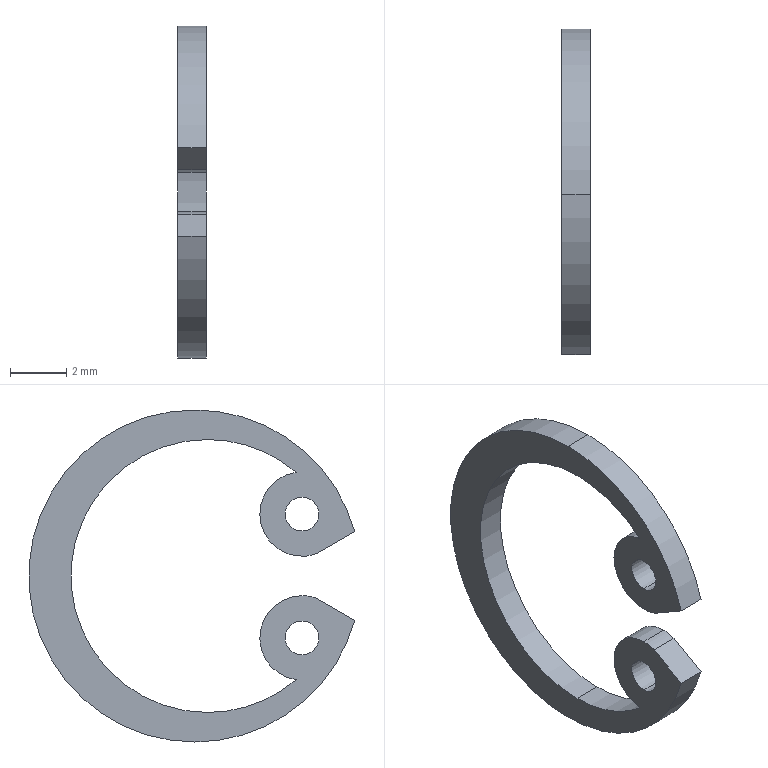Part | SolidWorks | features RefAxis 3, 3DProfileFeature 1, Extrusion 1 | 1 solid | 17 faces | box 1 x 11.586 x 11.8 mm | volume 42.993 mm3 | cylinder 13 | plane 4 | commonest cylinder face diameters 1.2 x4 3 x3 9.7 x3 11.8 x3
STEP:
#1=CARTESIAN_POINT('',(0.5,-3.811,2.8));
#2=VERTEX_POINT('',#1);
#3=CARTESIAN_POINT('',(0.5,-3.811,1.6));
#4=VERTEX_POINT('',#3);
#5=CARTESIAN_POINT('',(0.5,-3.811,2.2));
#6=DIRECTION('',(1.,0.,0.));
#7=DIRECTION('',(0.,0.,-1.));
#8=AXIS2_PLACEMENT_3D('',#5,#6,#7);
#9=CIRCLE('',#8,0.6);
#10=EDGE_CURVE('',#2,#4,#9,.T.);
#11=ORIENTED_EDGE('',*,*,#10,.T.);
#12=CARTESIAN_POINT('',(-0.5,-3.811,1.6));
#13=VERTEX_POINT('',#12);
#14=CARTESIAN_POINT('',(0.5,-3.811,1.6));
#15=DIRECTION('',(-1.,0.,0.));
#16=VECTOR('',#15,1000.);
#17=LINE('',#14,#16);
#18=EDGE_CURVE('',#4,#13,#17,.T.);
#19=ORIENTED_EDGE('',*,*,#18,.T.);
#20=CARTESIAN_POINT('',(-0.5,-3.811,2.8));
#21=VERTEX_POINT('',#20);
#22=CARTESIAN_POINT('',(-0.5,-3.811,2.2));
#23=DIRECTION('',(1.,0.,0.));
#24=DIRECTION('',(0.,0.,-1.));
#25=AXIS2_PLACEMENT_3D('',#22,#23,#24);
#26=CIRCLE('',#25,0.6);
#27=EDGE_CURVE('',#21,#13,#26,.T.);
#28=ORIENTED_EDGE('',*,*,#27,.F.);
#29=CARTESIAN_POINT('',(0.5,-3.811,2.8));
#30=DIRECTION('',(-1.,0.,0.));
#31=VECTOR('',#30,1000.);
#32=LINE('',#29,#31);
#33=EDGE_CURVE('',#2,#21,#32,.T.);
#34=ORIENTED_EDGE('',*,*,#33,.F.);
#35=EDGE_LOOP('',(#11,#19,#28,#34));
#36=FACE_OUTER_BOUND('',#35,.T.);
#37=CARTESIAN_POINT('',(0.5,-3.811,2.2));
#38=DIRECTION('',(-1.,0.,0.));
#39=DIRECTION('',(0.,0.,1.));
#40=AXIS2_PLACEMENT_3D('',#37,#38,#39);
#41=CYLINDRICAL_SURFACE('',#40,0.6);
#42=ADVANCED_FACE('',(#36),#41,.F.);
#43=CARTESIAN_POINT('',(0.5,-3.811,-1.6));
#44=VERTEX_POINT('',#43);
#45=CARTESIAN_POINT('',(0.5,-3.811,-2.8));
#46=VERTEX_POINT('',#45);
#47=CARTESIAN_POINT('',(0.5,-3.811,-2.2));
#48=DIRECTION('',(1.,0.,0.));
#49=DIRECTION('',(0.,0.,-1.));
#50=AXIS2_PLACEMENT_3D('',#47,#48,#49);
#51=CIRCLE('',#50,0.6);
#52=EDGE_CURVE('',#44,#46,#51,.T.);
#53=ORIENTED_EDGE('',*,*,#52,.T.);
#54=CARTESIAN_POINT('',(-0.5,-3.811,-2.8));
#55=VERTEX_POINT('',#54);
#56=CARTESIAN_POINT('',(0.5,-3.811,-2.8));
#57=DIRECTION('',(-1.,0.,0.));
#58=VECTOR('',#57,1000.);
#59=LINE('',#56,#58);
#60=EDGE_CURVE('',#46,#55,#59,.T.);
#61=ORIENTED_EDGE('',*,*,#60,.T.);
#62=CARTESIAN_POINT('',(-0.5,-3.811,-1.6));
#63=VERTEX_POINT('',#62);
#64=CARTESIAN_POINT('',(-0.5,-3.811,-2.2));
#65=DIRECTION('',(1.,0.,0.));
#66=DIRECTION('',(0.,0.,-1.));
#67=AXIS2_PLACEMENT_3D('',#64,#65,#66);
#68=CIRCLE('',#67,0.6);
#69=EDGE_CURVE('',#63,#55,#68,.T.);
#70=ORIENTED_EDGE('',*,*,#69,.F.);
#71=CARTESIAN_POINT('',(0.5,-3.811,-1.6));
#72=DIRECTION('',(-1.,0.,0.));
#73=VECTOR('',#72,1000.);
#74=LINE('',#71,#73);
#75=EDGE_CURVE('',#44,#63,#74,.T.);
#76=ORIENTED_EDGE('',*,*,#75,.F.);
#77=EDGE_LOOP('',(#53,#61,#70,#76));
#78=FACE_OUTER_BOUND('',#77,.T.);
#79=CARTESIAN_POINT('',(0.5,-3.811,-2.2));
#80=DIRECTION('',(-1.,0.,0.));
#81=DIRECTION('',(0.,0.,1.));
#82=AXIS2_PLACEMENT_3D('',#79,#80,#81);
#83=CYLINDRICAL_SURFACE('',#82,0.6);
#84=ADVANCED_FACE('',(#78),#83,.F.);
#85=CARTESIAN_POINT('',(0.5,-3.811,-0.7));
#86=VERTEX_POINT('',#85);
#87=CARTESIAN_POINT('',(0.5,-4.328,-0.7921));
#88=VERTEX_POINT('',#87);
#89=CARTESIAN_POINT('',(0.5,-3.811,-2.2));
#90=DIRECTION('',(1.,0.,0.));
#91=DIRECTION('',(0.,0.,-1.));
#92=AXIS2_PLACEMENT_3D('',#89,#90,#91);
#93=CIRCLE('',#92,1.5);
#94=EDGE_CURVE('',#86,#88,#93,.T.);
#95=ORIENTED_EDGE('',*,*,#94,.F.);
#96=CARTESIAN_POINT('',(-0.5,-3.811,-0.7));
#97=VERTEX_POINT('',#96);
#98=CARTESIAN_POINT('',(0.5,-3.811,-0.7));
#99=DIRECTION('',(-1.,0.,0.));
#100=VECTOR('',#99,1000.);
#101=LINE('',#98,#100);
#102=EDGE_CURVE('',#86,#97,#101,.T.);
#103=ORIENTED_EDGE('',*,*,#102,.T.);
#104=CARTESIAN_POINT('',(-0.5,-4.328,-0.7921));
#105=VERTEX_POINT('',#104);
#106=CARTESIAN_POINT('',(-0.5,-3.811,-2.2));
#107=DIRECTION('',(1.,0.,0.));
#108=DIRECTION('',(0.,0.,-1.));
#109=AXIS2_PLACEMENT_3D('',#106,#107,#108);
#110=CIRCLE('',#109,1.5);
#111=EDGE_CURVE('',#97,#105,#110,.T.);
#112=ORIENTED_EDGE('',*,*,#111,.T.);
#113=CARTESIAN_POINT('',(0.5,-4.328,-0.7921));
#114=DIRECTION('',(-1.,0.,0.));
#115=VECTOR('',#114,1000.);
#116=LINE('',#113,#115);
#117=EDGE_CURVE('',#88,#105,#116,.T.);
#118=ORIENTED_EDGE('',*,*,#117,.F.);
#119=EDGE_LOOP('',(#95,#103,#112,#118));
#120=FACE_OUTER_BOUND('',#119,.T.);
#121=CARTESIAN_POINT('',(0.5,-3.811,-2.2));
#122=DIRECTION('',(-1.,0.,0.));
#123=DIRECTION('',(0.,0.,1.));
#124=AXIS2_PLACEMENT_3D('',#121,#122,#123);
#125=CYLINDRICAL_SURFACE('',#124,1.5);
#126=ADVANCED_FACE('',(#120),#125,.T.);
#127=CARTESIAN_POINT('',(0.5,-0.45,-4.85));
#128=VERTEX_POINT('',#127);
#129=CARTESIAN_POINT('',(0.5,-3.603,-3.686));
#130=VERTEX_POINT('',#129);
#131=CARTESIAN_POINT('',(0.5,-0.45,0.));
#132=DIRECTION('',(-1.,0.,0.));
#133=DIRECTION('',(0.,0.,1.));
#134=AXIS2_PLACEMENT_3D('',#131,#132,#133);
#135=CIRCLE('',#134,4.85);
#136=EDGE_CURVE('',#128,#130,#135,.T.);
#137=ORIENTED_EDGE('',*,*,#136,.F.);
#138=CARTESIAN_POINT('',(-0.5,-0.45,-4.85));
#139=VERTEX_POINT('',#138);
#140=CARTESIAN_POINT('',(0.5,-0.45,-4.85));
#141=DIRECTION('',(-1.,0.,0.));
#142=VECTOR('',#141,1000.);
#143=LINE('',#140,#142);
#144=EDGE_CURVE('',#128,#139,#143,.T.);
#145=ORIENTED_EDGE('',*,*,#144,.T.);
#146=CARTESIAN_POINT('',(-0.5,-3.603,-3.686));
#147=VERTEX_POINT('',#146);
#148=CARTESIAN_POINT('',(-0.5,-0.45,0.));
#149=DIRECTION('',(-1.,0.,0.));
#150=DIRECTION('',(0.,0.,1.));
#151=AXIS2_PLACEMENT_3D('',#148,#149,#150);
#152=CIRCLE('',#151,4.85);
#153=EDGE_CURVE('',#139,#147,#152,.T.);
#154=ORIENTED_EDGE('',*,*,#153,.T.);
#155=CARTESIAN_POINT('',(0.5,-3.603,-3.686));
#156=DIRECTION('',(-1.,0.,0.));
#157=VECTOR('',#156,1000.);
#158=LINE('',#155,#157);
#159=EDGE_CURVE('',#130,#147,#158,.T.);
#160=ORIENTED_EDGE('',*,*,#159,.F.);
#161=EDGE_LOOP('',(#137,#145,#154,#160));
#162=FACE_OUTER_BOUND('',#161,.T.);
#163=CARTESIAN_POINT('',(0.5,-0.45,0.));
#164=DIRECTION('',(-1.,0.,0.));
#165=DIRECTION('',(0.,0.,1.));
#166=AXIS2_PLACEMENT_3D('',#163,#164,#165);
#167=CYLINDRICAL_SURFACE('',#166,4.85);
#168=ADVANCED_FACE('',(#162),#167,.F.);
#169=ORIENTED_EDGE('',*,*,#144,.F.);
#170=CARTESIAN_POINT('',(0.5,-0.45,4.85));
#171=VERTEX_POINT('',#170);
#172=CARTESIAN_POINT('',(0.5,-0.45,0.));
#173=DIRECTION('',(-1.,0.,0.));
#174=DIRECTION('',(0.,0.,1.));
#175=AXIS2_PLACEMENT_3D('',#172,#173,#174);
#176=CIRCLE('',#175,4.85);
#177=EDGE_CURVE('',#171,#128,#176,.T.);
#178=ORIENTED_EDGE('',*,*,#177,.F.);
#179=CARTESIAN_POINT('',(-0.5,-0.45,4.85));
#180=VERTEX_POINT('',#179);
#181=CARTESIAN_POINT('',(0.5,-0.45,4.85));
#182=DIRECTION('',(-1.,0.,0.));
#183=VECTOR('',#182,1000.);
#184=LINE('',#181,#183);
#185=EDGE_CURVE('',#171,#180,#184,.T.);
#186=ORIENTED_EDGE('',*,*,#185,.T.);
#187=CARTESIAN_POINT('',(-0.5,-0.45,0.));
#188=DIRECTION('',(-1.,0.,0.));
#189=DIRECTION('',(0.,0.,1.));
#190=AXIS2_PLACEMENT_3D('',#187,#188,#189);
#191=CIRCLE('',#190,4.85);
#192=EDGE_CURVE('',#180,#139,#191,.T.);
#193=ORIENTED_EDGE('',*,*,#192,.T.);
#194=EDGE_LOOP('',(#169,#178,#186,#193));
#195=FACE_OUTER_BOUND('',#194,.T.);
#196=CARTESIAN_POINT('',(0.5,-0.45,0.));
#197=DIRECTION('',(-1.,0.,0.));
#198=DIRECTION('',(0.,0.,1.));
#199=AXIS2_PLACEMENT_3D('',#196,#197,#198);
#200=CYLINDRICAL_SURFACE('',#199,4.85);
#201=ADVANCED_FACE('',(#195),#200,.F.);
#202=CARTESIAN_POINT('',(0.5,0.,-5.9));
#203=VERTEX_POINT('',#202);
#204=CARTESIAN_POINT('',(0.5,0.,5.9));
#205=VERTEX_POINT('',#204);
#206=CARTESIAN_POINT('',(0.5,0.,0.));
#207=DIRECTION('',(1.,0.,0.));
#208=DIRECTION('',(0.,0.,-1.));
#209=AXIS2_PLACEMENT_3D('',#206,#207,#208);
#210=CIRCLE('',#209,5.9);
#211=EDGE_CURVE('',#203,#205,#210,.T.);
#212=ORIENTED_EDGE('',*,*,#211,.F.);
#213=CARTESIAN_POINT('',(-0.5,0.,-5.9));
#214=VERTEX_POINT('',#213);
#215=CARTESIAN_POINT('',(0.5,0.,-5.9));
#216=DIRECTION('',(-1.,0.,0.));
#217=VECTOR('',#216,1000.);
#218=LINE('',#215,#217);
#219=EDGE_CURVE('',#203,#214,#218,.T.);
#220=ORIENTED_EDGE('',*,*,#219,.T.);
#221=CARTESIAN_POINT('',(-0.5,0.,5.9));
#222=VERTEX_POINT('',#221);
#223=CARTESIAN_POINT('',(-0.5,0.,0.));
#224=DIRECTION('',(1.,0.,0.));
#225=DIRECTION('',(0.,0.,-1.));
#226=AXIS2_PLACEMENT_3D('',#223,#224,#225);
#227=CIRCLE('',#226,5.9);
#228=EDGE_CURVE('',#214,#222,#227,.T.);
#229=ORIENTED_EDGE('',*,*,#228,.T.);
#230=CARTESIAN_POINT('',(0.5,0.,5.9));
#231=DIRECTION('',(-1.,0.,0.));
#232=VECTOR('',#231,1000.);
#233=LINE('',#230,#232);
#234=EDGE_CURVE('',#205,#222,#233,.T.);
#235=ORIENTED_EDGE('',*,*,#234,.F.);
#236=EDGE_LOOP('',(#212,#220,#229,#235));
#237=FACE_OUTER_BOUND('',#236,.T.);
#238=CARTESIAN_POINT('',(0.5,0.,0.));
#239=DIRECTION('',(-1.,0.,0.));
#240=DIRECTION('',(0.,0.,1.));
#241=AXIS2_PLACEMENT_3D('',#238,#239,#240);
#242=CYLINDRICAL_SURFACE('',#241,5.9);
#243=ADVANCED_FACE('',(#237),#242,.T.);
#244=CARTESIAN_POINT('',(0.5,-5.686,1.576));
#245=VERTEX_POINT('',#244);
#246=CARTESIAN_POINT('',(0.5,0.,0.));
#247=DIRECTION('',(1.,0.,0.));
#248=DIRECTION('',(0.,0.,-1.));
#249=AXIS2_PLACEMENT_3D('',#246,#247,#248);
#250=CIRCLE('',#249,5.9);
#251=EDGE_CURVE('',#205,#245,#250,.T.);
#252=ORIENTED_EDGE('',*,*,#251,.F.);
#253=ORIENTED_EDGE('',*,*,#234,.T.);
#254=CARTESIAN_POINT('',(-0.5,-5.686,1.576));
#255=VERTEX_POINT('',#254);
#256=CARTESIAN_POINT('',(-0.5,0.,0.));
#257=DIRECTION('',(1.,0.,0.));
#258=DIRECTION('',(0.,0.,-1.));
#259=AXIS2_PLACEMENT_3D('',#256,#257,#258);
#260=CIRCLE('',#259,5.9);
#261=EDGE_CURVE('',#222,#255,#260,.T.);
#262=ORIENTED_EDGE('',*,*,#261,.T.);
#263=CARTESIAN_POINT('',(0.5,-5.686,1.576));
#264=DIRECTION('',(-1.,0.,0.));
#265=VECTOR('',#264,1000.);
#266=LINE('',#263,#265);
#267=EDGE_CURVE('',#245,#255,#266,.T.);
#268=ORIENTED_EDGE('',*,*,#267,.F.);
#269=EDGE_LOOP('',(#252,#253,#262,#268));
#270=FACE_OUTER_BOUND('',#269,.T.);
#271=CARTESIAN_POINT('',(0.5,0.,0.));
#272=DIRECTION('',(-1.,0.,0.));
#273=DIRECTION('',(0.,0.,1.));
#274=AXIS2_PLACEMENT_3D('',#271,#272,#273);
#275=CYLINDRICAL_SURFACE('',#274,5.9);
#276=ADVANCED_FACE('',(#270),#275,.T.);
#277=ORIENTED_EDGE('',*,*,#52,.F.);
#278=CARTESIAN_POINT('',(0.5,-3.811,-2.2));
#279=DIRECTION('',(1.,0.,0.));
#280=DIRECTION('',(0.,0.,-1.));
#281=AXIS2_PLACEMENT_3D('',#278,#279,#280);
#282=CIRCLE('',#281,0.6);
#283=EDGE_CURVE('',#46,#44,#282,.T.);
#284=ORIENTED_EDGE('',*,*,#283,.F.);
#285=EDGE_LOOP('',(#277,#284));
#286=FACE_BOUND('',#285,.T.);
#287=CARTESIAN_POINT('',(0.5,-5.686,-1.576));
#288=VERTEX_POINT('',#287);
#289=CARTESIAN_POINT('',(0.5,0.,0.));
#290=DIRECTION('',(1.,0.,0.));
#291=DIRECTION('',(0.,0.,-1.));
#292=AXIS2_PLACEMENT_3D('',#289,#290,#291);
#293=CIRCLE('',#292,5.9);
#294=EDGE_CURVE('',#288,#203,#293,.T.);
#295=ORIENTED_EDGE('',*,*,#294,.T.);
#296=ORIENTED_EDGE('',*,*,#211,.T.);
#297=ORIENTED_EDGE('',*,*,#251,.T.);
#298=CARTESIAN_POINT('',(0.5,-4.328,0.7921));
#299=VERTEX_POINT('',#298);
#300=CARTESIAN_POINT('',(0.5,-5.686,1.576));
#301=DIRECTION('',(0.,0.866,-0.5));
#302=VECTOR('',#301,1000.);
#303=LINE('',#300,#302);
#304=EDGE_CURVE('',#245,#299,#303,.T.);
#305=ORIENTED_EDGE('',*,*,#304,.T.);
#306=CARTESIAN_POINT('',(0.5,-3.603,3.686));
#307=VERTEX_POINT('',#306);
#308=CARTESIAN_POINT('',(0.5,-3.811,2.2));
#309=DIRECTION('',(1.,0.,0.));
#310=DIRECTION('',(0.,0.,-1.));
#311=AXIS2_PLACEMENT_3D('',#308,#309,#310);
#312=CIRCLE('',#311,1.5);
#313=EDGE_CURVE('',#299,#307,#312,.T.);
#314=ORIENTED_EDGE('',*,*,#313,.T.);
#315=CARTESIAN_POINT('',(0.5,-0.45,0.));
#316=DIRECTION('',(-1.,0.,0.));
#317=DIRECTION('',(0.,0.,1.));
#318=AXIS2_PLACEMENT_3D('',#315,#316,#317);
#319=CIRCLE('',#318,4.85);
#320=EDGE_CURVE('',#307,#171,#319,.T.);
#321=ORIENTED_EDGE('',*,*,#320,.T.);
#322=ORIENTED_EDGE('',*,*,#177,.T.);
#323=ORIENTED_EDGE('',*,*,#136,.T.);
#324=CARTESIAN_POINT('',(0.5,-3.811,-2.2));
#325=DIRECTION('',(1.,0.,0.));
#326=DIRECTION('',(0.,0.,-1.));
#327=AXIS2_PLACEMENT_3D('',#324,#325,#326);
#328=CIRCLE('',#327,1.5);
#329=EDGE_CURVE('',#130,#86,#328,.T.);
#330=ORIENTED_EDGE('',*,*,#329,.T.);
#331=ORIENTED_EDGE('',*,*,#94,.T.);
#332=CARTESIAN_POINT('',(0.5,-4.328,-0.7921));
#333=DIRECTION('',(0.,-0.866,-0.5));
#334=VECTOR('',#333,1000.);
#335=LINE('',#332,#334);
#336=EDGE_CURVE('',#88,#288,#335,.T.);
#337=ORIENTED_EDGE('',*,*,#336,.T.);
#338=EDGE_LOOP('',(#295,#296,#297,#305,#314,#321,#322,#323,#330,#331,#337));
#339=FACE_OUTER_BOUND('',#338,.T.);
#340=ORIENTED_EDGE('',*,*,#10,.F.);
#341=CARTESIAN_POINT('',(0.5,-3.811,2.2));
#342=DIRECTION('',(1.,0.,0.));
#343=DIRECTION('',(0.,0.,-1.));
#344=AXIS2_PLACEMENT_3D('',#341,#342,#343);
#345=CIRCLE('',#344,0.6);
#346=EDGE_CURVE('',#4,#2,#345,.T.);
#347=ORIENTED_EDGE('',*,*,#346,.F.);
#348=EDGE_LOOP('',(#340,#347));
#349=FACE_BOUND('',#348,.T.);
#350=CARTESIAN_POINT('',(0.5,0.,0.));
#351=DIRECTION('',(1.,0.,0.));
#352=DIRECTION('',(0.,0.,-1.));
#353=AXIS2_PLACEMENT_3D('',#350,#351,#352);
#354=PLANE('',#353);
#355=ADVANCED_FACE('',(#286,#339,#349),#354,.T.);
#356=ORIENTED_EDGE('',*,*,#219,.F.);
#357=ORIENTED_EDGE('',*,*,#294,.F.);
#358=CARTESIAN_POINT('',(-0.5,-5.686,-1.576));
#359=VERTEX_POINT('',#358);
#360=CARTESIAN_POINT('',(0.5,-5.686,-1.576));
#361=DIRECTION('',(-1.,0.,0.));
#362=VECTOR('',#361,1000.);
#363=LINE('',#360,#362);
#364=EDGE_CURVE('',#288,#359,#363,.T.);
#365=ORIENTED_EDGE('',*,*,#364,.T.);
#366=CARTESIAN_POINT('',(-0.5,0.,0.));
#367=DIRECTION('',(1.,0.,0.));
#368=DIRECTION('',(0.,0.,-1.));
#369=AXIS2_PLACEMENT_3D('',#366,#367,#368);
#370=CIRCLE('',#369,5.9);
#371=EDGE_CURVE('',#359,#214,#370,.T.);
#372=ORIENTED_EDGE('',*,*,#371,.T.);
#373=EDGE_LOOP('',(#356,#357,#365,#372));
#374=FACE_OUTER_BOUND('',#373,.T.);
#375=CARTESIAN_POINT('',(0.5,0.,0.));
#376=DIRECTION('',(-1.,0.,0.));
#377=DIRECTION('',(0.,0.,1.));
#378=AXIS2_PLACEMENT_3D('',#375,#376,#377);
#379=CYLINDRICAL_SURFACE('',#378,5.9);
#380=ADVANCED_FACE('',(#374),#379,.T.);
#381=ORIENTED_EDGE('',*,*,#267,.T.);
#382=CARTESIAN_POINT('',(-0.5,-4.328,0.7921));
#383=VERTEX_POINT('',#382);
#384=CARTESIAN_POINT('',(-0.5,-5.686,1.576));
#385=DIRECTION('',(0.,0.866,-0.5));
#386=VECTOR('',#385,1000.);
#387=LINE('',#384,#386);
#388=EDGE_CURVE('',#255,#383,#387,.T.);
#389=ORIENTED_EDGE('',*,*,#388,.T.);
#390=CARTESIAN_POINT('',(0.5,-4.328,0.7921));
#391=DIRECTION('',(-1.,0.,0.));
#392=VECTOR('',#391,1000.);
#393=LINE('',#390,#392);
#394=EDGE_CURVE('',#299,#383,#393,.T.);
#395=ORIENTED_EDGE('',*,*,#394,.F.);
#396=ORIENTED_EDGE('',*,*,#304,.F.);
#397=EDGE_LOOP('',(#381,#389,#395,#396));
#398=FACE_OUTER_BOUND('',#397,.T.);
#399=CARTESIAN_POINT('',(0.5,-5.686,1.576));
#400=DIRECTION('',(0.,0.5,0.866));
#401=DIRECTION('',(0.,-0.866,0.5));
#402=AXIS2_PLACEMENT_3D('',#399,#400,#401);
#403=PLANE('',#402);
#404=ADVANCED_FACE('',(#398),#403,.F.);
#405=ORIENTED_EDGE('',*,*,#394,.T.);
#406=CARTESIAN_POINT('',(-0.5,-3.603,3.686));
#407=VERTEX_POINT('',#406);
#408=CARTESIAN_POINT('',(-0.5,-3.811,2.2));
#409=DIRECTION('',(1.,0.,0.));
#410=DIRECTION('',(0.,0.,-1.));
#411=AXIS2_PLACEMENT_3D('',#408,#409,#410);
#412=CIRCLE('',#411,1.5);
#413=EDGE_CURVE('',#383,#407,#412,.T.);
#414=ORIENTED_EDGE('',*,*,#413,.T.);
#415=CARTESIAN_POINT('',(0.5,-3.603,3.686));
#416=DIRECTION('',(-1.,0.,0.));
#417=VECTOR('',#416,1000.);
#418=LINE('',#415,#417);
#419=EDGE_CURVE('',#307,#407,#418,.T.);
#420=ORIENTED_EDGE('',*,*,#419,.F.);
#421=ORIENTED_EDGE('',*,*,#313,.F.);
#422=EDGE_LOOP('',(#405,#414,#420,#421));
#423=FACE_OUTER_BOUND('',#422,.T.);
#424=CARTESIAN_POINT('',(0.5,-3.811,2.2));
#425=DIRECTION('',(-1.,0.,0.));
#426=DIRECTION('',(0.,0.,1.));
#427=AXIS2_PLACEMENT_3D('',#424,#425,#426);
#428=CYLINDRICAL_SURFACE('',#427,1.5);
#429=ADVANCED_FACE('',(#423),#428,.T.);
#430=ORIENTED_EDGE('',*,*,#185,.F.);
#431=ORIENTED_EDGE('',*,*,#320,.F.);
#432=ORIENTED_EDGE('',*,*,#419,.T.);
#433=CARTESIAN_POINT('',(-0.5,-0.45,0.));
#434=DIRECTION('',(-1.,0.,0.));
#435=DIRECTION('',(0.,0.,1.));
#436=AXIS2_PLACEMENT_3D('',#433,#434,#435);
#437=CIRCLE('',#436,4.85);
#438=EDGE_CURVE('',#407,#180,#437,.T.);
#439=ORIENTED_EDGE('',*,*,#438,.T.);
#440=EDGE_LOOP('',(#430,#431,#432,#439));
#441=FACE_OUTER_BOUND('',#440,.T.);
#442=CARTESIAN_POINT('',(0.5,-0.45,0.));
#443=DIRECTION('',(-1.,0.,0.));
#444=DIRECTION('',(0.,0.,1.));
#445=AXIS2_PLACEMENT_3D('',#442,#443,#444);
#446=CYLINDRICAL_SURFACE('',#445,4.85);
#447=ADVANCED_FACE('',(#441),#446,.F.);
#448=ORIENTED_EDGE('',*,*,#102,.F.);
#449=ORIENTED_EDGE('',*,*,#329,.F.);
#450=ORIENTED_EDGE('',*,*,#159,.T.);
#451=CARTESIAN_POINT('',(-0.5,-3.811,-2.2));
#452=DIRECTION('',(1.,0.,0.));
#453=DIRECTION('',(0.,0.,-1.));
#454=AXIS2_PLACEMENT_3D('',#451,#452,#453);
#455=CIRCLE('',#454,1.5);
#456=EDGE_CURVE('',#147,#97,#455,.T.);
#457=ORIENTED_EDGE('',*,*,#456,.T.);
#458=EDGE_LOOP('',(#448,#449,#450,#457));
#459=FACE_OUTER_BOUND('',#458,.T.);
#460=CARTESIAN_POINT('',(0.5,-3.811,-2.2));
#461=DIRECTION('',(-1.,0.,0.));
#462=DIRECTION('',(0.,0.,1.));
#463=AXIS2_PLACEMENT_3D('',#460,#461,#462);
#464=CYLINDRICAL_SURFACE('',#463,1.5);
#465=ADVANCED_FACE('',(#459),#464,.T.);
#466=ORIENTED_EDGE('',*,*,#117,.T.);
#467=CARTESIAN_POINT('',(-0.5,-4.328,-0.7921));
#468=DIRECTION('',(0.,-0.866,-0.5));
#469=VECTOR('',#468,1000.);
#470=LINE('',#467,#469);
#471=EDGE_CURVE('',#105,#359,#470,.T.);
#472=ORIENTED_EDGE('',*,*,#471,.T.);
#473=ORIENTED_EDGE('',*,*,#364,.F.);
#474=ORIENTED_EDGE('',*,*,#336,.F.);
#475=EDGE_LOOP('',(#466,#472,#473,#474));
#476=FACE_OUTER_BOUND('',#475,.T.);
#477=CARTESIAN_POINT('',(0.5,-4.328,-0.7921));
#478=DIRECTION('',(0.,0.5,-0.866));
#479=DIRECTION('',(0.,0.866,0.5));
#480=AXIS2_PLACEMENT_3D('',#477,#478,#479);
#481=PLANE('',#480);
#482=ADVANCED_FACE('',(#476),#481,.F.);
#483=ORIENTED_EDGE('',*,*,#60,.F.);
#484=ORIENTED_EDGE('',*,*,#283,.T.);
#485=ORIENTED_EDGE('',*,*,#75,.T.);
#486=CARTESIAN_POINT('',(-0.5,-3.811,-2.2));
#487=DIRECTION('',(1.,0.,0.));
#488=DIRECTION('',(0.,0.,-1.));
#489=AXIS2_PLACEMENT_3D('',#486,#487,#488);
#490=CIRCLE('',#489,0.6);
#491=EDGE_CURVE('',#55,#63,#490,.T.);
#492=ORIENTED_EDGE('',*,*,#491,.F.);
#493=EDGE_LOOP('',(#483,#484,#485,#492));
#494=FACE_OUTER_BOUND('',#493,.T.);
#495=CARTESIAN_POINT('',(0.5,-3.811,-2.2));
#496=DIRECTION('',(-1.,0.,0.));
#497=DIRECTION('',(0.,0.,1.));
#498=AXIS2_PLACEMENT_3D('',#495,#496,#497);
#499=CYLINDRICAL_SURFACE('',#498,0.6);
#500=ADVANCED_FACE('',(#494),#499,.F.);
#501=ORIENTED_EDGE('',*,*,#18,.F.);
#502=ORIENTED_EDGE('',*,*,#346,.T.);
#503=ORIENTED_EDGE('',*,*,#33,.T.);
#504=CARTESIAN_POINT('',(-0.5,-3.811,2.2));
#505=DIRECTION('',(1.,0.,0.));
#506=DIRECTION('',(0.,0.,-1.));
#507=AXIS2_PLACEMENT_3D('',#504,#505,#506);
#508=CIRCLE('',#507,0.6);
#509=EDGE_CURVE('',#13,#21,#508,.T.);
#510=ORIENTED_EDGE('',*,*,#509,.F.);
#511=EDGE_LOOP('',(#501,#502,#503,#510));
#512=FACE_OUTER_BOUND('',#511,.T.);
#513=CARTESIAN_POINT('',(0.5,-3.811,2.2));
#514=DIRECTION('',(-1.,0.,0.));
#515=DIRECTION('',(0.,0.,1.));
#516=AXIS2_PLACEMENT_3D('',#513,#514,#515);
#517=CYLINDRICAL_SURFACE('',#516,0.6);
#518=ADVANCED_FACE('',(#512),#517,.F.);
#519=ORIENTED_EDGE('',*,*,#27,.T.);
#520=ORIENTED_EDGE('',*,*,#509,.T.);
#521=EDGE_LOOP('',(#519,#520));
#522=FACE_BOUND('',#521,.T.);
#523=ORIENTED_EDGE('',*,*,#69,.T.);
#524=ORIENTED_EDGE('',*,*,#491,.T.);
#525=EDGE_LOOP('',(#523,#524));
#526=FACE_BOUND('',#525,.T.);
#527=ORIENTED_EDGE('',*,*,#371,.F.);
#528=ORIENTED_EDGE('',*,*,#471,.F.);
#529=ORIENTED_EDGE('',*,*,#111,.F.);
#530=ORIENTED_EDGE('',*,*,#456,.F.);
#531=ORIENTED_EDGE('',*,*,#153,.F.);
#532=ORIENTED_EDGE('',*,*,#192,.F.);
#533=ORIENTED_EDGE('',*,*,#438,.F.);
#534=ORIENTED_EDGE('',*,*,#413,.F.);
#535=ORIENTED_EDGE('',*,*,#388,.F.);
#536=ORIENTED_EDGE('',*,*,#261,.F.);
#537=ORIENTED_EDGE('',*,*,#228,.F.);
#538=EDGE_LOOP('',(#527,#528,#529,#530,#531,#532,#533,#534,#535,#536,#537));
#539=FACE_OUTER_BOUND('',#538,.T.);
#540=CARTESIAN_POINT('',(-0.5,0.,0.));
#541=DIRECTION('',(1.,0.,0.));
#542=DIRECTION('',(0.,0.,-1.));
#543=AXIS2_PLACEMENT_3D('',#540,#541,#542);
#544=PLANE('',#543);
#545=ADVANCED_FACE('',(#522,#526,#539),#544,.F.);
#546=CLOSED_SHELL('',(#42,#84,#126,#168,#201,#243,#276,#355,#380,#404,#429,#447,#465,#482,#500,#518,#545));
#547=MANIFOLD_SOLID_BREP('',#546);
#548=CARTESIAN_POINT('',(0.,0.,0.));
#549=DIRECTION('',(0.,0.,1.));
#550=DIRECTION('',(1.,0.,0.));
#551=AXIS2_PLACEMENT_3D('',#548,#549,#550);
#552=(LENGTH_UNIT()NAMED_UNIT(*)SI_UNIT(.MILLI.,.METRE.));
#553=UNCERTAINTY_MEASURE_WITH_UNIT(LENGTH_MEASURE(0.00001),#552,'','');
#554=(NAMED_UNIT(*)PLANE_ANGLE_UNIT()SI_UNIT($,.RADIAN.));
#555=(NAMED_UNIT(*)SI_UNIT($,.STERADIAN.)SOLID_ANGLE_UNIT());
#556=(GEOMETRIC_REPRESENTATION_CONTEXT(3)GLOBAL_UNCERTAINTY_ASSIGNED_CONTEXT((#553))GLOBAL_UNIT_ASSIGNED_CONTEXT((#552,#554,#555))REPRESENTATION_CONTEXT('',''));
#557=ADVANCED_BREP_SHAPE_REPRESENTATION('',(#547,#551),#556);